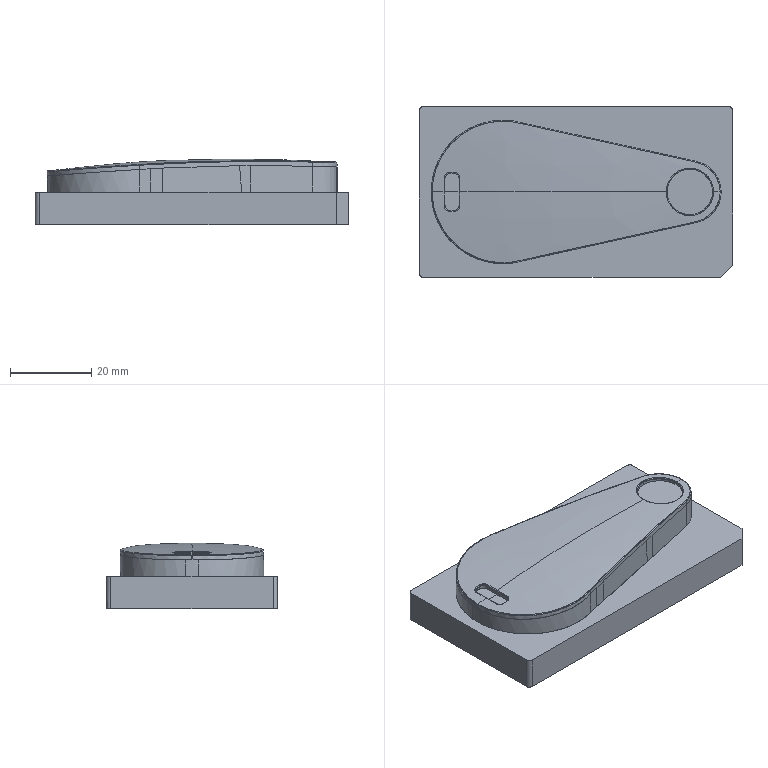NC program | PowerMill | posted with a generic post | part box 77 x 42 x 16.114 mm
Lines 1 to 934 of 230441:
%
O0001
N104 ( POWERMILL CB  : 2026004.0)
N105 ( POST VER      : 2026.0.0.5161)
N106 ( OPTION FILE   : FANUC)
N107 ( OUTPUT WORKPLANE : WORLD)
N108 (  )
N109 ( TOOL LIST )
N110 (---------------------------------------)
N111 ( NO. | ID        | DIA.| TIP RAD|LENGTH)
N112 (---------------------------------------)
N113 (    1|D10C_1_1   |10.0 |  0.0   |71.48 )
N114 (    2|D4C_1_1    | 4.0 |  0.0   |63.32 )
N115 (   28|D2C_1_1    | 2.0 |  0.0   |58.12 )
N116 (    3|D10_1_1    |10.0 |  0.0   | 71.2 )
N117 (    7|R2_1_1_1   | 4.0 |  2.0   |60.56 )
N118 (   12|D2_1_1     | 2.0 |  0.0   |58.28 )
N119 (    6|R0.5_1_1   | 1.0 |  0.5   |57.76 )
N120 (   13|TEXT_D4_1_1| 4.0 |  0.3   |63.36 )
N121 (---------------------------------------)
N122 (  )
N123 ( NUMBER OF TOOLPATHS: 15.0 )
N124 ( ESTIMATED PROGRAM DURATION: 0 HOURS 36 MIN 27 SEC)
N125 (  )
N126 G00 G21 G80 G40 G17
N127 G90
N128 G54
N129 G53 Z0.0
N130 (---------------)
N131 ( START TOOLPATH : 精公开粗01-扫面平行-D10C )
N132 (---------------)
N133 ( TOOL NO.    :1 )
N134 ( TOOL TYPE   : ENDMILL)
N135 ( TOOL ID     : D10C_1_1)
N136 ( TOOL DIA    : 10.0 LENGTH 71.48)
N137 T1
N138 M6
N139 S8000 M03
N140 G00 G90 X0.0 Y0.0
N141 G43 Z10.6 H1
N142
N143 G05 P10000 R4
N144 X46.28 Y23.78
N145 Z1.4665
N146 G01 Z0.2665 F6000.0
N147 X41.28 F10000.0
N148 X-41.28
N149 Y17.835
N150 X41.28
N151 Y11.89
N152 X-41.28
N153 Y5.945
N154 X41.28
N155 Y0.0
N156 X-41.28
N157 Y-5.945
N158 X41.28
N159 Y-11.89
N160 X-41.28
N161 Y-17.835
N162 X41.28
N163 Y-23.78
N164 X-41.28
N165 X-46.28
N166 Z-0.067
N167 X-41.28
N168 X41.28
N169 Y-17.835
N170 X-41.28
N171 Y-11.89
N172 X41.28
N173 Y-5.945
N174 X-41.28
N175 Y0.0
N176 X41.28
N177 Y5.945
N178 X-41.28
N179 Y11.89
N180 X41.28
N181 Y17.835
N182 X-41.28
N183 Y23.78
N184 X41.28
N185 X46.28
N186 G00 Z10.6
N187 G05 P0
N188 (---------------)
N189 ( END TOOLPATH : 精公开粗01-扫面平行-D10C )
N190 (---------------)
N191 ( START TOOLPATH : 精公开粗01-外形偏置-D10C )
N192 (---------------)
N193 G00 X0.0415 Y-0.002 Z9.883
N194 G05 P10000 R4
N195 X15.9242 Y-30.687
N196 Z0.7019
N197 G01 Z-0.4981 F6000.0
N198 Y-30.1595 F10000.0
N199 G03 X11.1767 Y-25.412 I-4.7475 J0.0
N200 G01 X-42.359
N201 G02 X-43.359 Y-24.412 I0.0 J1.0
N202 G01 Y-9.389
N203 X-38.1648
N204 X-32.274
N205 X-27.774
N206 X-32.274
N207 Y-12.327
N208 G03 X-30.3656 Y-14.3249 I2.0 J0.0
N209 G01 X-22.5359 Y-14.684
N210 G03 X-20.7651 Y-12.0881 I0.0846 J1.8442
N211 G01 X-21.6191 Y-10.1722
N212 G02 X-23.0394 Y5.7498 I22.5028 J10.0315
N213 G01 X-22.8829 Y6.3851
N214 X-22.7024 Y7.0728
N215 X-22.501 Y7.7546
N216 X-26.7967 Y9.0952
N217 X-22.501 Y7.7546
N218 G02 X-21.3301 Y10.7572 I22.2162 J-6.9337
N219 G01 X-20.7241 Y12.0408
N220 G03 X-22.4821 Y14.68 I-1.6738 J0.7902
N221 G01 X-30.365 Y14.3209
N222 G03 X-32.274 Y12.323 I0.091 J-1.9979
N223 G01 Y-9.389
N224 X-38.1648
N225 Y19.829
N226 G02 X-37.78 Y20.2138 I0.3848 J0.0
N227 G01 X-2.4368 Y20.2141
N228 G02 X-2.3958 Y19.9438 I0.0 J-0.1383
N229 G01 X-3.4127 Y19.6283
N230 G03 X-6.9587 Y18.12 I5.6371 J-18.1747
N231 G01 X-7.4423 Y17.8535
N232 G03 X-9.9489 Y16.16 I8.0696 J-14.6456
N233 G01 X-11.2345 Y15.1102
N234 G03 X-14.9934 Y10.7921 I10.7156 J-13.1228
N235 G01 X-15.4481 Y10.0446
N236 G03 X-17.8124 Y3.6108 I15.1633 J-9.2237
N237 G01 X-18.0077 Y2.3841
N238 G03 X-17.2464 Y-6.0193 I16.961 J-2.6996
N239 G01 X-16.8493 Y-7.1471
N240 G03 X-14.6778 Y-11.3148 I15.6839 J5.5221
N241 G01 X-14.3629 Y-11.754
N242 G03 X-10.8465 Y-15.4433 I14.9153 J10.6958
N243 G01 X-9.9392 Y-16.1623
N244 G03 X-4.3341 Y-19.2367 I11.8443 J14.9472
N245 G01 X-2.2596 Y-19.9548
N246 G02 X-2.3038 Y-20.2181 I-0.0442 J-0.1279
N247 G01 X-37.78 Y-20.2178
N248 G02 X-38.1648 Y-19.833 I0.0 J0.3848
N249 G01 Y-9.389
N250 X-43.359
N251 Y24.408
N252 G02 X-42.359 Y25.408 I1.0 J0.0
N253 G01 X42.442
N254 G02 X43.442 Y24.408 I0.0 J-1.0
N255 G01 Y-0.002
N256 X38.2478
N257 Y-19.833
N258 G02 X37.863 Y-20.2178 I-0.3848 J0.0
N259 G01 X21.0884 Y-20.2181
N260 G02 X21.0616 Y-19.967 I0.0 J0.127
N261 G01 X25.5196 Y-19.0042
N262 G03 X33.5356 Y-14.6039 I-3.3827 J15.6635
N263 G01 X34.141 Y-13.9894
N264 X34.9977 Y-13.0818
N265 G03 X37.2748 Y-9.4829 I-8.1466 J7.6745
N266 G01 X37.3311 Y-9.339
N267 G03 X37.0014 Y-1.3906 I-9.2052 J3.5992
N268 G01 X36.908 Y-1.2
N269 X36.7233 Y-0.8503
N270 X36.5177 Y-0.5124
N271 X36.4472 Y-0.4042
N272 G02 X36.4478 Y0.4116 I0.626 J0.4074
N273 G01 X36.5181 Y0.5193
N274 X36.7871 Y0.9702
N275 X37.0186 Y1.4415
N276 X37.0926 Y1.609
N277 X37.3321 Y2.1986
N278 X37.5356 Y2.8016
N279 X37.5738 Y2.9268
N280 G03 X37.7338 Y7.9564 I-9.2351 J2.8113
N281 G01 X37.6906 Y8.1397
N282 G03 X35.1378 Y12.9054 I-10.2377 J-2.4172
N283 G01 X34.0142 Y14.1076
N284 G03 X32.0914 Y15.8479 I-11.3514 J-10.6099
N285 G01 X31.5222 Y16.2824
N286 G03 X25.9999 Y18.8577 I-8.6385 J-11.3152
N287 G01 X22.0441 Y19.7452
N288 X21.0577 Y19.9635
N289 G02 X21.085 Y20.2141 I0.0273 J0.1238
N290 G01 X37.863 Y20.2138
N291 G02 X38.2478 Y19.829 I0.0 J-0.3848
N292 G01 Y-0.002
N293 X43.442
N294 Y-24.412
N295 G02 X42.442 Y-25.412 I-1.0 J0.0
N296 G01 X11.1767
N297 X10.8695 Y-16.6973
N298 X10.096 Y-16.7246
N299 X7.0023 Y-16.5623
N300 X6.2289 Y-16.464
N301 X4.6821 Y-16.2302
N302 X3.1352 Y-16.0073
N303 X1.5884 Y-15.7551
N304 X0.8149 Y-15.5221
N305 X-2.2788 Y-14.4397
N306 X-3.8256 Y-13.8544
N307 X-4.4213 Y-13.537
N308 X-5.3725 Y-12.9688
N309 X-6.6886 Y-11.9901
N310 X-8.4662 Y-10.5629
N311 X-8.6439 Y-10.4433
N312 X-9.2396 Y-9.8513
N313 X-10.013 Y-8.8847
N314 X-11.0312 Y-7.3496
N315 X-11.4723 Y-6.5761
N316 X-12.0853 Y-5.0293
N317 X-12.5796 Y-3.4824
N318 X-12.7465 Y-2.709
N319 X-12.9822 Y-0.3887
N320 X-13.0074 Y0.3847
N321 X-12.7744 Y1.9316
N322 X-12.5126 Y3.4784
N323 X-12.3333 Y4.351
N324 X-11.7762 Y5.7987
N325 X-11.5599 Y6.273
N326 X-10.7865 Y7.7151
N327 X-10.0019 Y8.8924
N328 X-9.4114 Y9.6658
N329 X-8.6577 Y10.4393
N330 X-6.9193 Y11.8759
N331 X-6.7451 Y11.9861
N332 X-6.1459 Y12.4686
N333 X-5.3725 Y13.0192
N334 X-4.5991 Y13.4836
N335 X-3.0522 Y14.1382
N336 X0.0415 Y15.3133
N337 X0.8149 Y15.5261
N338 X2.2794 Y15.8532
N339 X4.6821 Y16.2976
N340 X5.4555 Y16.3887
N341 X9.3226 Y16.708
N342 X10.8695 Y16.6997
N343 X11.4349 Y16.6267
N344 X13.9632 Y16.1719
N345 X17.0569 Y15.5309
N346 X22.4709 Y14.3165
N347 X24.7911 Y13.7425
N348 X26.338 Y13.2942
N349 X27.1114 Y12.9606
N350 X27.428 Y12.7595
N351 X28.5077 Y11.9861
N352 X29.4317 Y11.2879
N353 X30.2051 Y10.5775
N354 X30.3105 Y10.4393
N355 X30.9786 Y9.7466
N356 X31.752 Y8.8663
N357 X32.2019 Y8.119
N358 X32.5254 Y7.3313
N359 X32.7121 Y6.5721
N360 X32.7985 Y5.7987
N361 X32.7333 Y5.0253
N362 X32.5482 Y4.2518
N363 X32.239 Y3.4784
N364 X31.7557 Y2.705
N365 X31.0721 Y1.9316
N366 X31.0414 Y1.9194
N367 X30.9808 Y1.8906
N368 X30.9245 Y1.8539
N369 X30.2051 Y1.3124
N370 X29.929 Y1.1581
N371 X29.4317 Y0.9354
N372 X28.0631 Y0.4858
N373 X27.9698 Y0.4441
N374 X27.8869 Y0.3844
N375 X27.8742 Y0.3731
N376 G03 X27.871 Y-0.3713 I0.3323 J-0.3736
N377 G01 X27.8854 Y-0.3843
N378 X27.9702 Y-0.4461
N379 X28.0659 Y-0.4889
N380 X29.4317 Y-0.9341
N381 X29.9361 Y-1.1621
N382 X30.2051 Y-1.3097
N383 X30.9325 Y-1.8574
N384 X30.9802 Y-1.8892
N385 X31.0313 Y-1.9154
N386 X31.077 Y-1.9356
N387 X31.7651 Y-2.709
N388 X32.2432 Y-3.4824
N389 X32.5364 Y-4.2558
N390 X32.7342 Y-5.0293
N391 X32.7976 Y-5.8027
N392 X32.7413 Y-6.5761
N393 X32.514 Y-7.3496
N394 X32.2002 Y-8.123
N395 X31.7217 Y-8.8964
N396 X30.9786 Y-9.7698
N397 X30.3303 Y-10.4433
N398 X29.4317 Y-11.2888
N399 X27.4429 Y-12.7635
N400 X27.1114 Y-12.9622
N401 X26.338 Y-13.3025
N402 X24.0177 Y-13.9467
N403 X20.924 Y-14.6771
N404 X16.2835 Y-15.6979
N405 X13.9632 Y-16.1696
N406 X11.4285 Y-16.6307
N407 X10.8695 Y-16.6973
N408 X11.1767 Y-25.412
N409 G00 Z3.3208
N410 G01 X15.9242 Y-30.687
N411 G00 Z0.3208
N412 G01 Z-0.8792 F6000.0
N413 Y-30.1595 F10000.0
N414 G03 X11.1767 Y-25.412 I-4.7475 J0.0
N415 G01 X-28.5765
N416 X-28.7253 Y-20.6801
N417 X-28.9005 Y-15.1087
N418 G03 X-27.1408 Y-12.4415 I-0.0615 J1.9546
N419 G01 X-27.4619 Y-11.6169
N420 X-27.7136 Y-10.8955
N421 G02 X-29.2836 Y-4.248 I31.1075 J10.8558
N422 G01 X-29.3815 Y-3.488
N423 G02 X-27.6932 Y11.2364 I30.6401 J3.9458
N424 G01 X-27.2352 Y12.4666
N425 G03 X-29.5635 Y15.083 I-1.8572 J0.6914
N426 G01 X-31.1251 Y14.7008
N427 G03 X-32.6497 Y12.7581 I0.4754 J-1.9427
N428 G01 Y-12.7622
N429 G03 X-31.0519 Y-14.7213 I2.0 J0.0
N430 G01 X-29.3553 Y-15.0697
N431 X-29.1291 Y-15.1025
N432 X-28.9005 Y-15.1087
N433 X-28.7253 Y-20.6801
N434 X-36.5679 Y-20.6005
N435 G02 X-38.5476 Y-18.6006 I0.0203 J1.9999
N436 G01 Y18.5966
N437 G02 X-36.5679 Y20.5965 I2.0 J0.0
N438 G01 X-16.6268 Y20.7987
N439 G02 X-15.8347 Y18.7734 I0.0118 J-1.1629
N440 G01 X-16.3014 Y18.3512
N441 G03 X-24.052 Y0.1087 I15.8281 J-17.4926
N442 G01 X-24.0215 Y-0.8514
N443 G03 X-22.3796 Y-9.4198 I27.7925 J0.8839
N444 G01 X-22.2211 Y-9.8584
N445 X-21.9978 Y-10.3779
N446 G03 X-17.1329 Y-17.5766 I22.1553 J9.7296
N447 G01 X-15.8459 Y-18.832
N448 G02 X-16.6515 Y-20.8027 I-0.794 J-0.8254
N449 G01 X-28.7253 Y-20.6801
N450 X-28.5765 Y-25.412
N451 X-42.359
N452 G02 X-43.359 Y-24.412 I0.0 J1.0
N453 G01 Y24.408
N454 G02 X-42.359 Y25.408 I1.0 J0.0
N455 G01 X23.2697
N456 X23.2002 Y20.7995
N457 X36.6608 Y20.5964
N458 G02 X38.6207 Y18.7951 I-0.0302 J-1.9998
N459 G01 X38.8247 Y16.7497
N460 G02 X36.6949 Y15.2528 I-1.4867 J-0.1483
N461 G01 X35.2486 Y15.9425
N462 G03 X23.8444 Y18.9702 I-13.7718 J-28.8807
N463 G01 X23.121 Y19.0239
N464 G02 X23.2002 Y20.7995 I0.0658 J0.8866
N465 G01 X23.2697 Y25.408
N466 X42.442
N467 G02 X43.442 Y24.408 I0.0 J-1.0
N468 G01 Y0.8369
N469 X40.7739 Y0.6747
N470 X40.7915 Y0.3847
N471 X40.7848 Y-0.3887
N472 X40.7441 Y-1.1621
N473 X40.6515 Y-1.9356
N474 X40.5119 Y-2.709
N475 X40.3243 Y-3.4824
N476 X40.0851 Y-4.2558
N477 X39.7923 Y-5.0293
N478 X39.4387 Y-5.8027
N479 X38.7128 Y-7.0849
N480 X37.9394 Y-8.1575
N481 X37.2991 Y-8.8964
N482 X36.5041 Y-9.6698
N483 X35.6191 Y-10.397
N484 X34.8457 Y-10.9291
N485 X34.3685 Y-11.2167
N486 X33.2988 Y-11.7688
N487 X32.7869 Y-11.9901
N488 X31.752 Y-12.3609
N489 X30.9786 Y-12.5757
N490 X5.6026 Y-18.1775
N491 X1.9469 Y-18.9509
N492 X-1.5054 Y-19.581
N493 X-2.2788 Y-19.6697
N494 X-3.0522 Y-19.7222
N495 X-3.8256 Y-19.6822
N496 X-4.5991 Y-19.5038
N497 X-6.9193 Y-18.7232
N498 X-7.6928 Y-18.4223
N499 X-8.4662 Y-18.0527
N500 X-9.7207 Y-17.4041
N501 X-12.3333 Y-15.6829
N502 X-13.1068 Y-15.0629
N503 X-13.8971 Y-14.3104
N504 X-14.5589 Y-13.537
N505 X-14.6536 Y-13.3899
N506 X-15.787 Y-11.9901
N507 X-16.2005 Y-11.4389
N508 X-16.7852 Y-10.4433
N509 X-17.6324 Y-8.8964
N510 X-17.9588 Y-8.123
N511 X-18.1745 Y-7.3496
N512 X-18.6765 Y-5.8027
N513 X-18.9967 Y-4.2558
N514 X-19.2586 Y-2.709
N515 X-19.3555 Y-1.1621
N516 X-19.4529 Y-0.3887
N517 X-19.4519 Y0.3847
N518 X-19.1654 Y3.4784
N519 X-19.0515 Y4.2518
N520 X-18.5207 Y6.2001
N521 X-18.1538 Y7.3456
N522 X-18.1494 Y7.3637
N523 X-17.9681 Y8.119
N524 X-17.7473 Y8.6584
N525 X-16.9739 Y10.1893
N526 X-16.349 Y11.2127
N527 X-15.2357 Y12.7595
N528 X-13.8802 Y14.3189
N529 X-13.0912 Y15.0798
N530 X-12.3333 Y15.6813
N531 X-10.9588 Y16.6267
N532 X-9.702 Y17.4001
N533 X-7.6928 Y18.4289
N534 X-6.9193 Y18.725
N535 X-4.5991 Y19.5117
N536 X-3.8256 Y19.6769
N537 X-3.0522 Y19.7213
N538 X-2.2788 Y19.6706
N539 X-1.5054 Y19.5818
N540 X1.9689 Y18.9469
N541 X5.6321 Y18.1735
N542 X30.9786 Y12.5746
N543 X31.752 Y12.3607
N544 X32.5254 Y12.0881
N545 X33.2988 Y11.7686
N546 X34.0723 Y11.3828
N547 X34.8457 Y10.9293
N548 X35.5564 Y10.4393
N549 X36.3925 Y9.7691
N550 X37.166 Y9.0356
N551 X37.9666 Y8.119
N552 X38.7128 Y7.0846
N553 X39.4407 Y5.7987
N554 X39.7936 Y5.0253
N555 X40.0858 Y4.2518
N556 X40.2597 Y3.7099
N557 X40.5137 Y2.705
N558 X40.6522 Y1.9316
N559 X40.7445 Y1.1581
N560 X40.7739 Y0.6747
N561 X43.442 Y0.8369
N562 Y-17.2101
N563 X38.8247 Y-16.7503
N564 X38.6208 Y-18.7988
N565 G02 X36.6609 Y-20.6004 I-1.9902 J0.1982
N566 G01 X23.2348 Y-20.8035
N567 G02 X23.0297 Y-19.0498 I-0.0135 J0.8873
N568 G01 X31.9511 Y-17.076
N569 X32.3692 Y-16.9678
N570 G03 X35.4282 Y-15.8512 I-4.4308 J16.8868
N571 G01 X36.6936 Y-15.2502
N572 G02 X38.8247 Y-16.7503 I0.642 J-1.3519
N573 G01 X43.442 Y-17.2101
N574 Y-24.412
N575 G02 X42.442 Y-25.412 I-1.0 J0.0
N576 G01 X11.1767
N577 G00 Z2.9397
N578 G01 X15.9242 Y-30.687
N579 G00 Z-0.0603
N580 G01 Z-1.2603 F6000.0
N581 Y-30.1595 F10000.0
N582 G03 X11.1767 Y-25.412 I-4.7475 J0.0
N583 G01 X-42.359
N584 G02 X-43.359 Y-24.412 I0.0 J1.0
N585 G01 Y-12.3437
N586 X-38.5476 Y-12.2891
N587 X-33.9136 Y-12.2365
N588 X-33.8881 Y-14.4836
N589 G03 X-32.1883 Y-15.9352 I1.4841 J0.0168
N590 G03 X-30.9779 Y-14.056 I-0.2157 J1.4684
N591 G01 X-31.7869 Y-11.2471
N592 X-32.1885 Y-9.7528
N593 G03 X-33.9391 Y-9.9895 I-0.8607 J-0.2266
N594 G01 X-33.9136 Y-12.2365
N595 X-38.5476 Y-12.2891
N596 Y18.5966
N597 G02 X-36.5799 Y20.5964 I2.0 J0.0
N598 G01 X-24.0887 Y20.7982
N599 G02 X-22.9742 Y18.678 I0.0216 J-1.3417
N600 G01 X-23.532 Y17.895
N601 G03 X-27.1857 Y10.8407 I23.0053 J-16.3887
N602 G01 X-31.6085 Y12.2064
N603 X-32.1745 Y10.3733
N604 G02 X-33.9391 Y10.6434 I-0.8622 J0.2662
N605 G01 X-33.9227 Y14.4804
N606 G02 X-32.2269 Y15.93 I1.4729 J-0.0063
N607 G02 X-31.0425 Y14.0395 I-0.2229 J-1.4559
N608 G01 X-31.6085 Y12.2064
N609 X-27.1857 Y10.8407
N610 G03 X-28.7706 Y1.1712 I26.659 J-9.3343
N611 G01 X-28.7505 Y-0.5261
N612 G03 X-27.8413 Y-8.0795 I35.3114 J0.4191
N613 G01 X-27.7152 Y-8.6233
N614 G03 X-23.7592 Y-17.528 I25.0859 J5.8136
N615 G01 X-22.967 Y-18.6653
N616 G02 X-24.1048 Y-20.8021 I-1.1158 J-0.7772
N617 G01 X-36.58 Y-20.6004
N618 G02 X-38.5476 Y-18.6006 I0.0324 J1.9998
N619 G01 Y-12.2891
N620 X-43.359 Y-12.3437
N621 Y24.408
N622 G02 X-42.359 Y25.408 I1.0 J0.0
N623 G01 X23.335
N624 X23.2651 Y20.7995
N625 X36.6609 Y20.5964
N626 G02 X38.6203 Y18.7998 I-0.0303 J-1.9998
N627 G01 X38.8243 Y16.8013
N628 G02 X36.6905 Y15.2902 I-1.4939 J-0.1525
N629 G01 X35.2392 Y15.9738
N630 G03 X23.9114 Y18.9688 I-13.8144 J-29.329
N631 G01 X23.1835 Y19.0248
N632 G02 X23.2651 Y20.7995 I0.0682 J0.8861
N633 G01 X23.335 Y25.408
N634 X42.442
N635 G02 X43.442 Y24.408 I0.0 J-1.0
N636 G01 Y0.83
N637 X40.8905 Y0.6747
N638 X40.9082 Y0.3847
N639 X40.9094 Y-0.3887
N640 X40.8633 Y-1.1621
N641 X40.7696 Y-1.9356
N642 X40.6238 Y-2.709
N643 X40.4364 Y-3.4824
N644 X40.2597 Y-4.0606
N645 X39.896 Y-5.0293
N646 X39.5373 Y-5.8027
N647 X39.1178 Y-6.5761
N648 X38.7128 Y-7.2251
N649 X38.0511 Y-8.123
N650 X37.3756 Y-8.8964
N651 X36.5787 Y-9.6698
N652 X35.6209 Y-10.4433
N653 X34.8457 Y-10.97
N654 X34.0723 Y-11.4151
N655 X32.8544 Y-11.9901
N656 X31.752 Y-12.3818
N657 X30.9786 Y-12.59
N658 X-2.2788 Y-19.9252
N659 X-6.9193 Y-20.9126
N660 X-8.9766 Y-21.2712
N661 X-10.013 Y-21.3871
N662 X-10.7865 Y-21.4115
N663 X-11.5599 Y-21.3532
N664 X-12.3333 Y-21.1717
N665 X-13.1068 Y-20.8599
N666 X-13.8802 Y-20.4429
N667 X-15.075 Y-19.7244
N668 X-16.9739 Y-18.2901
N669 X-18.6862 Y-16.6307
N670 X-19.3387 Y-15.8572
N671 X-20.4029 Y-14.3104
N672 X-20.8666 Y-13.537
N673 X-21.2855 Y-12.7635
N674 X-22.3879 Y-10.2129
N675 X-22.7937 Y-8.8964
N676 X-23.0828 Y-8.123
N677 X-23.2873 Y-7.3496
N678 X-23.7348 Y-5.0293
N679 X-24.0044 Y-2.709
N680 X-24.1307 Y-0.3887
N681 X-24.1312 Y0.3847
N682 X-24.0634 Y1.1581
N683 X-24.063 Y1.1648
N684 X-23.9224 Y3.4784
N685 X-23.8267 Y4.2518
N686 X-23.5643 Y5.7987
N687 X-23.4028 Y6.5721
N688 X-23.277 Y7.3456
N689 X-22.842 Y8.8924
N690 X-22.3879 Y10.1634
N691 X-21.9973 Y11.2127
N692 X-21.2881 Y12.7595
N693 X-20.4126 Y14.3064
N694 X-19.8782 Y15.0798
N695 X-19.2945 Y15.8532
N696 X-18.6375 Y16.6267
N697 X-17.7473 Y17.56
N698 X-17.118 Y18.1735
N699 X-16.2005 Y18.935
N700 X-15.427 Y19.4646
N701 X-14.6536 Y19.9373
N702 X-13.1068 Y20.8566
N703 X-12.3333 Y21.1754
N704 X-11.5599 Y21.3525
N705 X-10.7865 Y21.4127
N706 X-10.013 Y21.3886
N707 X-9.2396 Y21.3125
N708 X-7.6928 Y21.0557
N709 X-6.1459 Y20.7548
N710 X-0.7319 Y19.5861
N711 X30.9786 Y12.5901
N712 X31.752 Y12.3818
N713 X32.8638 Y11.9861
N714 X34.0723 Y11.4152
N715 X34.8457 Y10.97
N716 X35.6191 Y10.4445
N717 X36.3925 Y9.8292
N718 X37.166 Y9.1079
N719 X37.9394 Y8.2562
N720 X38.6294 Y7.3456
N721 X39.1186 Y6.5721
N722 X39.4863 Y5.9007
N723 X39.8962 Y5.0253
N724 X40.1972 Y4.2518
N725 X40.4377 Y3.4784
N726 X40.6284 Y2.705
N727 X40.7684 Y1.9316
N728 X40.8611 Y1.1581
N729 X40.8905 Y0.6747
N730 X43.442 Y0.83
N731 Y-17.2802
N732 X38.8244 Y-16.808
N733 X38.6202 Y-18.8041
N734 G02 X36.661 Y-20.6004 I-1.9896 J0.2035
N735 G01 X23.2909 Y-20.8035
N736 G02 X23.086 Y-19.05 I-0.0135 J0.8872
N737 G01 X31.7702 Y-17.1313
N738 G03 X35.1783 Y-15.9966 I-3.733 J16.8965
N739 G01 X36.7235 Y-15.2965
N740 G02 X38.8244 Y-16.808 I0.616 J-1.3596
N741 G01 X43.442 Y-17.2802
N742 Y-24.412
N743 G02 X42.442 Y-25.412 I-1.0 J0.0
N744 G01 X11.1767
N745 G00 Z2.5586
N746 G01 X15.9242 Y-30.687
N747 G00 Z-0.4414
N748 G01 Z-1.6414 F6000.0
N749 Y-30.1595 F10000.0
N750 G03 X11.1767 Y-25.412 I-4.7475 J0.0
N751 G01 X-42.359
N752 G02 X-43.359 Y-24.412 I0.0 J1.0
N753 G01 Y24.408
N754 G02 X-42.359 Y25.408 I1.0 J0.0
N755 G01 X23.3991
N756 X23.3289 Y20.7995
N757 X36.6611 Y20.5964
N758 G02 X38.6201 Y18.8015 I-0.0305 J-1.9998
N759 G01 X38.8242 Y16.8192
N760 G02 X36.6727 Y15.3161 I-1.4934 J-0.1538
N761 G01 X35.0745 Y16.0955
N762 G03 X23.957 Y18.9856 I-12.7077 J-26.0553
N763 G01 X23.2666 Y19.0235
N764 G02 X23.3289 Y20.7995 I0.0487 J0.8874
N765 G01 X23.3991 Y25.408
N766 X42.442
N767 G02 X43.442 Y24.408 I0.0 J-1.0
N768 G01 Y0.8209
N769 X40.904 Y0.6747
N770 X40.9207 Y0.3847
N771 Y-0.3887
N772 X40.8773 Y-1.1621
N773 X40.7829 Y-1.9356
N774 X40.6385 Y-2.709
N775 X40.4512 Y-3.4824
N776 X40.2107 Y-4.2558
N777 X39.9095 Y-5.0293
N778 X39.5512 Y-5.8027
N779 X39.1334 Y-6.5761
N780 X38.7128 Y-7.2489
N781 X38.0682 Y-8.123
N782 X37.3938 Y-8.8964
N783 X36.5988 Y-9.6698
N784 X35.6437 Y-10.4433
N785 X34.8457 Y-10.9857
N786 X34.0723 Y-11.4304
N787 X32.89 Y-11.9901
N788 X31.752 Y-12.3959
N789 X31.0454 Y-12.5719
N790 X30.9785 Y-12.5899
N791 X30.932 Y-12.6002
N792 X30.2766 Y-12.7635
N793 X29.7296 Y-12.884
N794 X30.7174 Y-17.3716
N795 X31.8049 Y-17.1322
N796 G03 X35.1912 Y-16.0058 I-3.6798 J16.7166
N797 G01 X36.7228 Y-15.3116
N798 G02 X38.8242 Y-16.8245 I0.6163 J-1.3598
N799 G01 X38.6201 Y-18.8056
N800 G02 X36.661 Y-20.6004 I-1.9895 J0.205
N801 G01 X23.3097 Y-20.8035
N802 G02 X23.1052 Y-19.0473 I-0.0135 J0.8885
N803 G01 X30.7174 Y-17.3716
N804 X29.7296 Y-12.884
N805 X-11.8804 Y-22.0447
N806 X-11.8825 Y-22.0451
N807 X-13.1068 Y-22.3258
N808 X-13.8802 Y-22.4577
N809 X-15.427 Y-22.6071
N810 X-16.2005 Y-22.6198
N811 X-16.9739 Y-22.5544
N812 X-17.7473 Y-22.4219
N813 X-18.5207 Y-22.1709
N814 X-18.8208 Y-22.0447
N815 X-19.2942 Y-21.7807
N816 X-19.9787 Y-21.2712
N817 X-20.9112 Y-20.4978
N818 X-21.6144 Y-19.8596
N819 X-22.4349 Y-18.9509
N820 X-23.6221 Y-17.4041
N821 X-23.9347 Y-16.9387
N822 X-24.5837 Y-15.8572
N823 X-24.979 Y-15.0838
N824 X-25.4816 Y-13.9134
N825 X-25.9554 Y-12.7635
N826 X-26.255 Y-11.9491
N827 X-26.3725 Y-11.5615
N828 X-30.7281 Y-12.9976
N829 G03 X-29.4585 Y-16.3276 I36.9855 J12.1945
N830 G01 X-29.2415 Y-16.8269
N831 X-28.3515 Y-18.6448
N832 G02 X-29.7361 Y-20.8015 I-1.3407 J-0.6621
N833 G01 X-36.6063 Y-20.5998
N834 G02 X-38.5476 Y-18.6006 I0.0587 J1.9992
N835 G01 Y18.5966
N836 G02 X-36.6065 Y20.5957 I2.0 J0.0
N837 G01 X-29.7552 Y20.7974
N838 G02 X-28.3542 Y18.5936 I0.0447 J-1.5188
N839 G01 X-29.0633 Y17.1897
N840 G03 X-32.7593 Y0.0435 I30.9856 J-15.6507
N841 G01 X-32.6505 Y-2.4805
N842 G03 X-30.7281 Y-12.9976 I38.909 J1.6778
N843 G01 X-26.3725 Y-11.5615
N844 X-26.9459 Y-9.6698
N845 X-27.4485 Y-7.3496
N846 X-27.7956 Y-5.0293
N847 X-27.8729 Y-4.2558
N848 X-28.0399 Y-1.9356
N849 X-28.0842 Y-0.3887
N850 X-28.0766 Y0.3847
N851 X-27.9459 Y3.4784
N852 X-27.5627 Y6.5721
N853 X-27.4347 Y7.3456
N854 X-26.9469 Y9.6658
N855 X-26.7302 Y10.4393
N856 X-26.247 Y11.9861
N857 X-25.6598 Y13.533
N858 X-24.7081 Y15.5944
N859 X-23.9347 Y16.9509
N860 X-23.6469 Y17.4001
N861 X-23.082 Y18.1735
N862 X-22.4619 Y18.9469
N863 X-21.712 Y19.7204
N864 X-20.0676 Y21.1997
N865 X-19.2942 Y21.7748
N866 X-18.8219 Y22.0407
N867 X-18.5207 Y22.1787
N868 X-17.7473 Y22.4243
N869 X-16.9739 Y22.5551
N870 X-16.2005 Y22.6193
N871 X-15.427 Y22.6068
N872 X-14.6536 Y22.5464
N873 X-13.8802 Y22.4547
N874 X-13.1068 Y22.3254
N875 X-11.8671 Y22.0407
N876 X0.0415 Y19.43
N877 X30.9786 Y12.6038
N878 X31.752 Y12.3959
N879 X32.8988 Y11.9861
N880 X34.0723 Y11.4304
N881 X34.8457 Y10.9859
N882 X35.6191 Y10.4608
N883 X36.3925 Y9.8464
N884 X37.166 Y9.1263
N885 X37.9394 Y8.2764
N886 X38.6458 Y7.3456
N887 X39.1347 Y6.5721
N888 X39.4863 Y5.9303
N889 X39.9105 Y5.0253
N890 X40.2121 Y4.2518
N891 X40.4525 Y3.4784
N892 X40.6389 Y2.705
N893 X40.7824 Y1.9316
N894 X40.8762 Y1.1581
N895 X40.904 Y0.6747
N896 X43.442 Y0.8209
N897 Y-24.412
N898 G02 X42.442 Y-25.412 I-1.0 J0.0
N899 G01 X11.1767
N900 G00 Z2.1775
N901 G01 X15.9242 Y-30.687
N902 G00 Z-0.8225
N903 G01 Z-2.0225 F6000.0
N904 Y-30.1595 F10000.0
N905 G03 X11.1767 Y-25.412 I-4.7475 J0.0
N906 G01 X-42.359
N907 G02 X-43.359 Y-24.412 I0.0 J1.0
N908 G01 Y24.408
N909 G02 X-42.359 Y25.408 I1.0 J0.0
N910 G01 X23.4382
N911 X23.3678 Y20.7995
N912 X36.6612 Y20.5964
N913 G02 X38.6199 Y18.8029 I-0.0306 J-1.9998
N914 G01 X38.8241 Y16.834
N915 G02 X36.6892 Y15.3201 I-1.4944 J-0.155
N916 G01 X35.1997 Y16.0221
N917 G03 X24.0093 Y18.9698 I-13.5632 J-28.7754
N918 G01 X23.2879 Y19.0238
N919 G02 X23.3678 Y20.7995 I0.0663 J0.8866
N920 G01 X23.4382 Y25.408
N921 X42.442
N922 G02 X43.442 Y24.408 I0.0 J-1.0
N923 G01 Y0.8223
N924 X40.9188 Y0.6747
N925 X40.9357 Y0.3847
N926 X40.9328 Y-0.3887
N927 X40.8907 Y-1.1621
N928 X40.7962 Y-1.9356
N929 X40.6534 Y-2.709
N930 X40.466 Y-3.4824
N931 X40.2247 Y-4.2558
N932 X39.9246 Y-5.0293
N933 X39.5652 Y-5.8027
N934 X39.1491 Y-6.5761
N935 X38.7128 Y-7.2726
N936 X38.0853 Y-8.123
N937 X37.412 Y-8.8964
N938 X36.6189 Y-9.6698
N939 X35.6661 Y-10.4433
N940 X34.8457 Y-11.0004
N941 X34.0723 Y-11.4441
N942 X32.9198 Y-11.9901
N943 X31.752 Y-12.4066
N944 X30.9786 Y-12.6138
N945 X2.3618 Y-18.9344
N946 X-11.5599 Y-21.9839
N947 X-11.5665 Y-21.9856
N948 X-13.1068 Y-22.3672
N949 X-14.6536 Y-22.6418
N950 X-16.2904 Y-22.8181
N951 X-17.7473 Y-22.8762
N952 X-19.2942 Y-22.8261
N953 X-20.841 Y-22.6548
N954 X-21.6144 Y-22.5175
N955 X-22.3879 Y-22.3466
N956 X-23.1613 Y-22.1406
N957 X-23.9347 Y-21.8712
N958 X-24.7081 Y-21.5144
N959 X-25.1472 Y-21.2712
N960 X-25.4816 Y-21.0485
N961 X-26.255 Y-20.3559
N962 X-27.0284 Y-19.3418
N963 X-27.7562 Y-18.1775
N964 X-28.1567 Y-17.4041
N965 X-28.9086 Y-15.8572
N966 X-29.5026 Y-14.3104
N967 X-29.9753 Y-12.7993
N968 X-34.3531 Y-14.1051
N969 X-33.9524 Y-15.3851
N970 X-33.5171 Y-16.6538
N971 X-33.259 Y-17.3742
N972 X-32.7434 Y-18.6951
N973 G02 X-34.1816 Y-20.706 I-1.3738 J-0.5372
N974 G01 X-36.635 Y-20.5987
N975 G02 X-38.5476 Y-18.6006 I0.0874 J1.9981
N976 G01 Y18.5966
N977 G02 X-36.724 Y20.5888 I2.0 J0.0
N978 G01 X-34.4332 Y20.7916
N979 G02 X-32.7894 Y18.5618 I0.143 J-1.6153
N980 G01 X-33.4618 Y16.9194
N981 G03 X-36.0529 Y6.3311 I34.0686 J-13.948
N982 G01 X-36.2135 Y4.5785
N983 G03 X-34.3531 Y-14.1051 I49.3392 J-4.5217
N984 G01 X-29.9753 Y-12.7993
N985 X-29.9865 Y-12.7635
N986 X-30.4142 Y-11.2167
N987 X-30.9285 Y-8.8964
N988 X-31.3101 Y-6.5761
N989 X-31.5772 Y-4.2558
N990 X-31.669 Y-2.7756
N991 X-31.7602 Y-0.3887
N992 X-31.7217 Y1.9316
N993 X-31.643 Y3.4784
N994 X-31.3046 Y6.5721
N995 X-30.8956 Y9.083
N996 X-30.4143 Y11.2127
N997 X-29.988 Y12.7595
N998 X-29.5056 Y14.3064
N999 X-28.9167 Y15.8532
N1000 X-28.1749 Y17.4001
N1001 X-27.7476 Y18.1735
N1002 X-27.2763 Y18.9469
N1003 X-26.7586 Y19.7204
N1004 X-26.255 Y20.3653
N1005 X-25.4816 Y21.0473
N1006 X-25.153 Y21.2672
N1007 X-24.7081 Y21.513
N1008 X-23.9347 Y21.8633
N1009 X-23.4717 Y22.0407
N1010 X-22.3879 Y22.3467
N1011 X-21.6144 Y22.5209
N1012 X-20.841 Y22.6565
N1013 X-20.0676 Y22.7571
N1014 X-18.5207 Y22.8672
N1015 X-17.7473 Y22.8728
N1016 X-16.2005 Y22.8093
N1017 X-14.6536 Y22.6398
N1018 X-13.1068 Y22.3672
N1019 X-11.8072 Y22.0407
N1020 X0.8149 Y19.274
N1021 X30.9786 Y12.6135
N1022 X31.752 Y12.4067
N1023 X32.9281 Y11.9861
N1024 X34.0723 Y11.4441
N1025 X34.8457 Y11.0006
N1026 X35.6715 Y10.4393
N1027 X36.3925 Y9.8637
N1028 X37.166 Y9.1464
N1029 X37.9394 Y8.2953
N1030 X38.6621 Y7.3456
N1031 X39.1508 Y6.5721